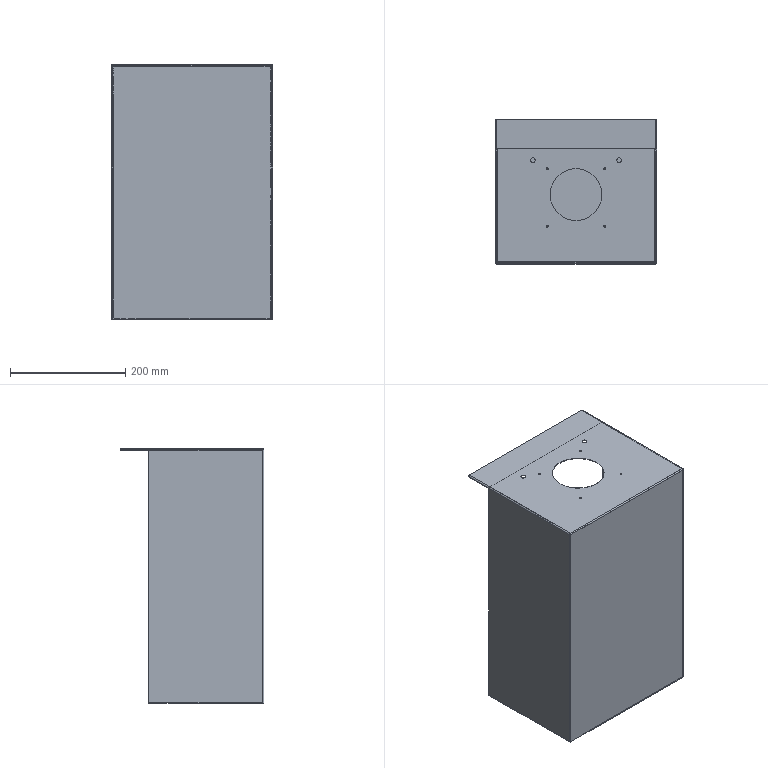Part | NX | 1 solid | 50 faces | box 280 x 250 x 443 mm | volume 446416 mm3 | cylinder 24 | plane 14 | cone 8 | sphere 4 | commonest cylinder face diameters 4 x10 2.5 x8 8.2 x4 90 x2
STEP:
#1=CARTESIAN_POINT('',(140.,100.,447.));
#2=VERTEX_POINT('',#1);
#3=CARTESIAN_POINT('',(140.,100.,7.));
#4=VERTEX_POINT('',#3);
#5=CARTESIAN_POINT('',(140.,100.,0.));
#6=DIRECTION('',(0.,0.,-1.));
#7=VECTOR('',#6,1000.);
#8=LINE('',#5,#7);
#9=EDGE_CURVE('',#2,#4,#8,.T.);
#10=ORIENTED_EDGE('',*,*,#9,.T.);
#11=CARTESIAN_POINT('',(-140.,100.,7.));
#12=VERTEX_POINT('',#11);
#13=CARTESIAN_POINT('',(0.,100.,7.));
#14=DIRECTION('',(-1.,0.,0.));
#15=VECTOR('',#14,1000.);
#16=LINE('',#13,#15);
#17=EDGE_CURVE('',#4,#12,#16,.T.);
#18=ORIENTED_EDGE('',*,*,#17,.T.);
#19=CARTESIAN_POINT('',(-140.,100.,447.));
#20=VERTEX_POINT('',#19);
#21=CARTESIAN_POINT('',(-140.,100.,0.));
#22=DIRECTION('',(0.,0.,-1.));
#23=VECTOR('',#22,1000.);
#24=LINE('',#21,#23);
#25=EDGE_CURVE('',#20,#12,#24,.T.);
#26=ORIENTED_EDGE('',*,*,#25,.F.);
#27=CARTESIAN_POINT('',(-139.,100.,447.));
#28=VERTEX_POINT('',#27);
#29=CARTESIAN_POINT('',(-140.,100.,447.));
#30=DIRECTION('',(1.,0.,0.));
#31=VECTOR('',#30,1000.);
#32=LINE('',#29,#31);
#33=EDGE_CURVE('',#20,#28,#32,.T.);
#34=ORIENTED_EDGE('',*,*,#33,.T.);
#35=CARTESIAN_POINT('',(-139.,100.,8.));
#36=VERTEX_POINT('',#35);
#37=CARTESIAN_POINT('',(-139.,100.,0.));
#38=DIRECTION('',(0.,0.,-1.));
#39=VECTOR('',#38,1000.);
#40=LINE('',#37,#39);
#41=EDGE_CURVE('',#28,#36,#40,.T.);
#42=ORIENTED_EDGE('',*,*,#41,.T.);
#43=CARTESIAN_POINT('',(139.,100.,8.));
#44=VERTEX_POINT('',#43);
#45=CARTESIAN_POINT('',(0.,100.,8.));
#46=DIRECTION('',(-1.,0.,0.));
#47=VECTOR('',#46,1000.);
#48=LINE('',#45,#47);
#49=EDGE_CURVE('',#44,#36,#48,.T.);
#50=ORIENTED_EDGE('',*,*,#49,.F.);
#51=CARTESIAN_POINT('',(139.,100.,447.));
#52=VERTEX_POINT('',#51);
#53=CARTESIAN_POINT('',(139.,100.,0.));
#54=DIRECTION('',(0.,0.,-1.));
#55=VECTOR('',#54,1000.);
#56=LINE('',#53,#55);
#57=EDGE_CURVE('',#52,#44,#56,.T.);
#58=ORIENTED_EDGE('',*,*,#57,.F.);
#59=CARTESIAN_POINT('',(139.,100.,447.));
#60=DIRECTION('',(1.,0.,0.));
#61=VECTOR('',#60,1000.);
#62=LINE('',#59,#61);
#63=EDGE_CURVE('',#52,#2,#62,.T.);
#64=ORIENTED_EDGE('',*,*,#63,.T.);
#65=EDGE_LOOP('',(#10,#18,#26,#34,#42,#50,#58,#64));
#66=FACE_BOUND('',#65,.T.);
#67=CARTESIAN_POINT('',(140.,100.,0.));
#68=DIRECTION('',(0.,1.,0.));
#69=DIRECTION('',(1.,0.,0.));
#70=AXIS2_PLACEMENT_3D('',#67,#68,#69);
#71=PLANE('',#70);
#72=ADVANCED_FACE('',(#66),#71,.T.);
#73=ORIENTED_EDGE('',*,*,#63,.F.);
#74=CARTESIAN_POINT('',(-139.,100.,447.));
#75=DIRECTION('',(1.,0.,0.));
#76=VECTOR('',#75,1000.);
#77=LINE('',#74,#76);
#78=EDGE_CURVE('',#28,#52,#77,.T.);
#79=ORIENTED_EDGE('',*,*,#78,.F.);
#80=ORIENTED_EDGE('',*,*,#33,.F.);
#81=CARTESIAN_POINT('',(-140.,150.,447.));
#82=VERTEX_POINT('',#81);
#83=CARTESIAN_POINT('',(-140.,150.,447.));
#84=DIRECTION('',(0.,-1.,0.));
#85=VECTOR('',#84,1000.);
#86=LINE('',#83,#85);
#87=EDGE_CURVE('',#82,#20,#86,.T.);
#88=ORIENTED_EDGE('',*,*,#87,.F.);
#89=CARTESIAN_POINT('',(140.,150.,447.));
#90=VERTEX_POINT('',#89);
#91=CARTESIAN_POINT('',(-140.,150.,447.));
#92=DIRECTION('',(1.,0.,0.));
#93=VECTOR('',#92,1000.);
#94=LINE('',#91,#93);
#95=EDGE_CURVE('',#82,#90,#94,.T.);
#96=ORIENTED_EDGE('',*,*,#95,.T.);
#97=CARTESIAN_POINT('',(140.,150.,447.));
#98=DIRECTION('',(0.,-1.,0.));
#99=VECTOR('',#98,1000.);
#100=LINE('',#97,#99);
#101=EDGE_CURVE('',#90,#2,#100,.T.);
#102=ORIENTED_EDGE('',*,*,#101,.T.);
#103=EDGE_LOOP('',(#73,#79,#80,#88,#96,#102));
#104=FACE_BOUND('',#103,.T.);
#105=CARTESIAN_POINT('',(140.,100.,447.));
#106=DIRECTION('',(0.,0.,-1.));
#107=DIRECTION('',(0.,-1.,0.));
#108=AXIS2_PLACEMENT_3D('',#105,#106,#107);
#109=PLANE('',#108);
#110=ADVANCED_FACE('',(#104),#109,.T.);
#111=CARTESIAN_POINT('',(-139.,-97.,447.));
#112=VERTEX_POINT('',#111);
#113=CARTESIAN_POINT('',(-139.,100.,447.));
#114=DIRECTION('',(0.,-1.,0.));
#115=VECTOR('',#114,1000.);
#116=LINE('',#113,#115);
#117=EDGE_CURVE('',#28,#112,#116,.T.);
#118=ORIENTED_EDGE('',*,*,#117,.T.);
#119=CARTESIAN_POINT('',(-139.,-97.,8.));
#120=VERTEX_POINT('',#119);
#121=CARTESIAN_POINT('',(-139.,-97.,447.));
#122=DIRECTION('',(0.,0.,-1.));
#123=VECTOR('',#122,1000.);
#124=LINE('',#121,#123);
#125=EDGE_CURVE('',#112,#120,#124,.T.);
#126=ORIENTED_EDGE('',*,*,#125,.T.);
#127=CARTESIAN_POINT('',(-139.,0.,8.));
#128=DIRECTION('',(0.,-1.,0.));
#129=VECTOR('',#128,1000.);
#130=LINE('',#127,#129);
#131=EDGE_CURVE('',#36,#120,#130,.T.);
#132=ORIENTED_EDGE('',*,*,#131,.F.);
#133=ORIENTED_EDGE('',*,*,#41,.F.);
#134=EDGE_LOOP('',(#118,#126,#132,#133));
#135=FACE_BOUND('',#134,.T.);
#136=CARTESIAN_POINT('',(-139.,100.,0.));
#137=DIRECTION('',(-1.,0.,0.));
#138=DIRECTION('',(0.,0.,1.));
#139=AXIS2_PLACEMENT_3D('',#136,#137,#138);
#140=PLANE('',#139);
#141=ADVANCED_FACE('',(#135),#140,.F.);
#142=CARTESIAN_POINT('',(139.,-97.,447.));
#143=VERTEX_POINT('',#142);
#144=CARTESIAN_POINT('',(139.,-97.,447.));
#145=DIRECTION('',(0.,1.,0.));
#146=VECTOR('',#145,1000.);
#147=LINE('',#144,#146);
#148=EDGE_CURVE('',#143,#52,#147,.T.);
#149=ORIENTED_EDGE('',*,*,#148,.T.);
#150=ORIENTED_EDGE('',*,*,#57,.T.);
#151=CARTESIAN_POINT('',(139.,-97.,8.));
#152=VERTEX_POINT('',#151);
#153=CARTESIAN_POINT('',(139.,0.,8.));
#154=DIRECTION('',(0.,1.,0.));
#155=VECTOR('',#154,1000.);
#156=LINE('',#153,#155);
#157=EDGE_CURVE('',#152,#44,#156,.T.);
#158=ORIENTED_EDGE('',*,*,#157,.F.);
#159=CARTESIAN_POINT('',(139.,-97.,3.));
#160=DIRECTION('',(0.,0.,1.));
#161=VECTOR('',#160,1000.);
#162=LINE('',#159,#161);
#163=EDGE_CURVE('',#152,#143,#162,.T.);
#164=ORIENTED_EDGE('',*,*,#163,.T.);
#165=EDGE_LOOP('',(#149,#150,#158,#164));
#166=FACE_BOUND('',#165,.T.);
#167=CARTESIAN_POINT('',(139.,-100.,0.));
#168=DIRECTION('',(1.,0.,0.));
#169=DIRECTION('',(0.,1.,0.));
#170=AXIS2_PLACEMENT_3D('',#167,#168,#169);
#171=PLANE('',#170);
#172=ADVANCED_FACE('',(#166),#171,.F.);
#173=CARTESIAN_POINT('',(137.,100.,449.));
#174=VERTEX_POINT('',#173);
#175=CARTESIAN_POINT('',(137.,100.,447.));
#176=DIRECTION('',(0.,1.,0.));
#177=DIRECTION('',(0.,0.,1.));
#178=AXIS2_PLACEMENT_3D('',#175,#176,#177);
#179=CIRCLE('',#178,2.);
#180=EDGE_CURVE('',#174,#52,#179,.T.);
#181=ORIENTED_EDGE('',*,*,#180,.T.);
#182=ORIENTED_EDGE('',*,*,#148,.F.);
#183=CARTESIAN_POINT('',(137.,-97.,449.));
#184=VERTEX_POINT('',#183);
#185=CARTESIAN_POINT('',(137.,-97.,447.));
#186=DIRECTION('',(0.,1.,0.));
#187=DIRECTION('',(1.,0.,0.));
#188=AXIS2_PLACEMENT_3D('',#185,#186,#187);
#189=CIRCLE('',#188,2.);
#190=EDGE_CURVE('',#184,#143,#189,.T.);
#191=ORIENTED_EDGE('',*,*,#190,.F.);
#192=CARTESIAN_POINT('',(137.,100.,449.));
#193=DIRECTION('',(0.,-1.,0.));
#194=VECTOR('',#193,1000.);
#195=LINE('',#192,#194);
#196=EDGE_CURVE('',#174,#184,#195,.T.);
#197=ORIENTED_EDGE('',*,*,#196,.F.);
#198=EDGE_LOOP('',(#181,#182,#191,#197));
#199=FACE_BOUND('',#198,.T.);
#200=CARTESIAN_POINT('',(137.,-99.854,447.));
#201=DIRECTION('',(0.,1.,0.));
#202=DIRECTION('',(0.,0.,1.));
#203=AXIS2_PLACEMENT_3D('',#200,#201,#202);
#204=CYLINDRICAL_SURFACE('',#203,2.);
#205=ADVANCED_FACE('',(#199),#204,.F.);
#206=CARTESIAN_POINT('',(138.,-100.,7.));
#207=VERTEX_POINT('',#206);
#208=CARTESIAN_POINT('',(138.,-100.,448.));
#209=VERTEX_POINT('',#208);
#210=CARTESIAN_POINT('',(138.,-100.,2.));
#211=DIRECTION('',(0.,0.,1.));
#212=VECTOR('',#211,1000.);
#213=LINE('',#210,#212);
#214=EDGE_CURVE('',#207,#209,#213,.T.);
#215=ORIENTED_EDGE('',*,*,#214,.F.);
#216=CARTESIAN_POINT('',(140.,-98.,7.));
#217=VERTEX_POINT('',#216);
#218=CARTESIAN_POINT('',(138.,-98.,7.));
#219=DIRECTION('',(0.,0.,-1.));
#220=DIRECTION('',(1.,0.,0.));
#221=AXIS2_PLACEMENT_3D('',#218,#219,#220);
#222=CIRCLE('',#221,2.);
#223=EDGE_CURVE('',#217,#207,#222,.T.);
#224=ORIENTED_EDGE('',*,*,#223,.F.);
#225=CARTESIAN_POINT('',(140.,-98.,448.));
#226=VERTEX_POINT('',#225);
#227=CARTESIAN_POINT('',(140.,-98.,448.));
#228=DIRECTION('',(0.,0.,-1.));
#229=VECTOR('',#228,1000.);
#230=LINE('',#227,#229);
#231=EDGE_CURVE('',#226,#217,#230,.T.);
#232=ORIENTED_EDGE('',*,*,#231,.F.);
#233=CARTESIAN_POINT('',(138.,-98.,448.));
#234=DIRECTION('',(0.,0.,-1.));
#235=DIRECTION('',(1.,0.,0.));
#236=AXIS2_PLACEMENT_3D('',#233,#234,#235);
#237=CIRCLE('',#236,2.);
#238=EDGE_CURVE('',#226,#209,#237,.T.);
#239=ORIENTED_EDGE('',*,*,#238,.T.);
#240=EDGE_LOOP('',(#215,#224,#232,#239));
#241=FACE_BOUND('',#240,.T.);
#242=CARTESIAN_POINT('',(138.,-98.,450.886));
#243=DIRECTION('',(0.,0.,-1.));
#244=DIRECTION('',(1.,0.,0.));
#245=AXIS2_PLACEMENT_3D('',#242,#243,#244);
#246=CYLINDRICAL_SURFACE('',#245,2.);
#247=ADVANCED_FACE('',(#241),#246,.T.);
#248=CARTESIAN_POINT('',(-140.,-98.,7.));
#249=VERTEX_POINT('',#248);
#250=CARTESIAN_POINT('',(-140.,-98.,448.));
#251=VERTEX_POINT('',#250);
#252=CARTESIAN_POINT('',(-140.,-98.,2.));
#253=DIRECTION('',(0.,0.,1.));
#254=VECTOR('',#253,1000.);
#255=LINE('',#252,#254);
#256=EDGE_CURVE('',#249,#251,#255,.T.);
#257=ORIENTED_EDGE('',*,*,#256,.F.);
#258=CARTESIAN_POINT('',(-138.,-100.,7.));
#259=VERTEX_POINT('',#258);
#260=CARTESIAN_POINT('',(-138.,-98.,7.));
#261=DIRECTION('',(0.,0.,-1.));
#262=DIRECTION('',(0.,-1.,0.));
#263=AXIS2_PLACEMENT_3D('',#260,#261,#262);
#264=CIRCLE('',#263,2.);
#265=EDGE_CURVE('',#259,#249,#264,.T.);
#266=ORIENTED_EDGE('',*,*,#265,.F.);
#267=CARTESIAN_POINT('',(-138.,-100.,448.));
#268=VERTEX_POINT('',#267);
#269=CARTESIAN_POINT('',(-138.,-100.,448.));
#270=DIRECTION('',(0.,0.,-1.));
#271=VECTOR('',#270,1000.);
#272=LINE('',#269,#271);
#273=EDGE_CURVE('',#268,#259,#272,.T.);
#274=ORIENTED_EDGE('',*,*,#273,.F.);
#275=CARTESIAN_POINT('',(-138.,-98.,448.));
#276=DIRECTION('',(0.,0.,-1.));
#277=DIRECTION('',(0.,-1.,0.));
#278=AXIS2_PLACEMENT_3D('',#275,#276,#277);
#279=CIRCLE('',#278,2.);
#280=EDGE_CURVE('',#268,#251,#279,.T.);
#281=ORIENTED_EDGE('',*,*,#280,.T.);
#282=EDGE_LOOP('',(#257,#266,#274,#281));
#283=FACE_BOUND('',#282,.T.);
#284=CARTESIAN_POINT('',(-138.,-98.,450.886));
#285=DIRECTION('',(0.,0.,-1.));
#286=DIRECTION('',(0.,-1.,0.));
#287=AXIS2_PLACEMENT_3D('',#284,#285,#286);
#288=CYLINDRICAL_SURFACE('',#287,2.);
#289=ADVANCED_FACE('',(#283),#288,.T.);
#290=CARTESIAN_POINT('',(-138.,-98.,450.));
#291=VERTEX_POINT('',#290);
#292=CARTESIAN_POINT('',(-138.,-98.,448.));
#293=DIRECTION('',(1.,0.,0.));
#294=DIRECTION('',(0.,0.,1.));
#295=AXIS2_PLACEMENT_3D('',#292,#293,#294);
#296=CIRCLE('',#295,2.);
#297=EDGE_CURVE('',#291,#268,#296,.T.);
#298=ORIENTED_EDGE('',*,*,#297,.F.);
#299=CARTESIAN_POINT('',(-138.,-98.,448.));
#300=DIRECTION('',(0.,1.,0.));
#301=DIRECTION('',(1.,0.,0.));
#302=AXIS2_PLACEMENT_3D('',#299,#300,#301);
#303=CIRCLE('',#302,2.);
#304=EDGE_CURVE('',#251,#291,#303,.T.);
#305=ORIENTED_EDGE('',*,*,#304,.F.);
#306=ORIENTED_EDGE('',*,*,#280,.F.);
#307=EDGE_LOOP('',(#298,#305,#306));
#308=FACE_BOUND('',#307,.T.);
#309=CARTESIAN_POINT('',(-138.,-98.,448.));
#310=DIRECTION('',(0.,1.,0.));
#311=DIRECTION('',(1.,0.,0.));
#312=AXIS2_PLACEMENT_3D('',#309,#310,#311);
#313=SPHERICAL_SURFACE('',#312,2.);
#314=ADVANCED_FACE('',(#308),#313,.T.);
#315=CARTESIAN_POINT('',(-140.,150.,448.));
#316=VERTEX_POINT('',#315);
#317=CARTESIAN_POINT('',(-140.,-98.,448.));
#318=DIRECTION('',(0.,1.,0.));
#319=VECTOR('',#318,1000.);
#320=LINE('',#317,#319);
#321=EDGE_CURVE('',#251,#316,#320,.T.);
#322=ORIENTED_EDGE('',*,*,#321,.F.);
#323=ORIENTED_EDGE('',*,*,#304,.T.);
#324=CARTESIAN_POINT('',(-138.,150.,450.));
#325=VERTEX_POINT('',#324);
#326=CARTESIAN_POINT('',(-138.,150.,450.));
#327=DIRECTION('',(0.,-1.,0.));
#328=VECTOR('',#327,1000.);
#329=LINE('',#326,#328);
#330=EDGE_CURVE('',#325,#291,#329,.T.);
#331=ORIENTED_EDGE('',*,*,#330,.F.);
#332=CARTESIAN_POINT('',(-138.,150.,448.));
#333=DIRECTION('',(0.,-1.,0.));
#334=DIRECTION('',(0.,0.,1.));
#335=AXIS2_PLACEMENT_3D('',#332,#333,#334);
#336=CIRCLE('',#335,2.);
#337=EDGE_CURVE('',#325,#316,#336,.T.);
#338=ORIENTED_EDGE('',*,*,#337,.T.);
#339=EDGE_LOOP('',(#322,#323,#331,#338));
#340=FACE_BOUND('',#339,.T.);
#341=CARTESIAN_POINT('',(-138.,100.871,448.));
#342=DIRECTION('',(0.,-1.,0.));
#343=DIRECTION('',(0.,0.,1.));
#344=AXIS2_PLACEMENT_3D('',#341,#342,#343);
#345=CYLINDRICAL_SURFACE('',#344,2.);
#346=ADVANCED_FACE('',(#340),#345,.T.);
#347=CARTESIAN_POINT('',(140.,150.,448.));
#348=VERTEX_POINT('',#347);
#349=CARTESIAN_POINT('',(138.,150.,450.));
#350=VERTEX_POINT('',#349);
#351=CARTESIAN_POINT('',(138.,150.,448.));
#352=DIRECTION('',(0.,-1.,0.));
#353=DIRECTION('',(1.,0.,0.));
#354=AXIS2_PLACEMENT_3D('',#351,#352,#353);
#355=CIRCLE('',#354,2.);
#356=EDGE_CURVE('',#348,#350,#355,.T.);
#357=ORIENTED_EDGE('',*,*,#356,.F.);
#358=CARTESIAN_POINT('',(140.,150.,447.));
#359=DIRECTION('',(0.,0.,1.));
#360=VECTOR('',#359,1000.);
#361=LINE('',#358,#360);
#362=EDGE_CURVE('',#90,#348,#361,.T.);
#363=ORIENTED_EDGE('',*,*,#362,.F.);
#364=ORIENTED_EDGE('',*,*,#95,.F.);
#365=CARTESIAN_POINT('',(-140.,150.,448.));
#366=DIRECTION('',(0.,0.,-1.));
#367=VECTOR('',#366,1000.);
#368=LINE('',#365,#367);
#369=EDGE_CURVE('',#316,#82,#368,.T.);
#370=ORIENTED_EDGE('',*,*,#369,.F.);
#371=ORIENTED_EDGE('',*,*,#337,.F.);
#372=CARTESIAN_POINT('',(0.,150.,450.));
#373=DIRECTION('',(1.,0.,0.));
#374=VECTOR('',#373,1000.);
#375=LINE('',#372,#374);
#376=EDGE_CURVE('',#325,#350,#375,.T.);
#377=ORIENTED_EDGE('',*,*,#376,.T.);
#378=EDGE_LOOP('',(#357,#363,#364,#370,#371,#377));
#379=FACE_BOUND('',#378,.T.);
#380=CARTESIAN_POINT('',(0.,150.,0.));
#381=DIRECTION('',(0.,1.,0.));
#382=DIRECTION('',(1.,0.,0.));
#383=AXIS2_PLACEMENT_3D('',#380,#381,#382);
#384=PLANE('',#383);
#385=ADVANCED_FACE('',(#379),#384,.T.);
#386=CARTESIAN_POINT('',(138.,-98.,450.));
#387=VERTEX_POINT('',#386);
#388=CARTESIAN_POINT('',(-138.,-98.,450.));
#389=DIRECTION('',(1.,0.,0.));
#390=VECTOR('',#389,1000.);
#391=LINE('',#388,#390);
#392=EDGE_CURVE('',#291,#387,#391,.T.);
#393=ORIENTED_EDGE('',*,*,#392,.F.);
#394=ORIENTED_EDGE('',*,*,#297,.T.);
#395=CARTESIAN_POINT('',(138.,-100.,448.));
#396=DIRECTION('',(-1.,0.,0.));
#397=VECTOR('',#396,1000.);
#398=LINE('',#395,#397);
#399=EDGE_CURVE('',#209,#268,#398,.T.);
#400=ORIENTED_EDGE('',*,*,#399,.F.);
#401=CARTESIAN_POINT('',(138.,-98.,448.));
#402=DIRECTION('',(-1.,0.,0.));
#403=DIRECTION('',(0.,-1.,0.));
#404=AXIS2_PLACEMENT_3D('',#401,#402,#403);
#405=CIRCLE('',#404,2.);
#406=EDGE_CURVE('',#209,#387,#405,.T.);
#407=ORIENTED_EDGE('',*,*,#406,.T.);
#408=EDGE_LOOP('',(#393,#394,#400,#407));
#409=FACE_BOUND('',#408,.T.);
#410=CARTESIAN_POINT('',(-140.871,-98.,448.));
#411=DIRECTION('',(1.,0.,0.));
#412=DIRECTION('',(0.,0.,1.));
#413=AXIS2_PLACEMENT_3D('',#410,#411,#412);
#414=CYLINDRICAL_SURFACE('',#413,2.);
#415=ADVANCED_FACE('',(#409),#414,.T.);
#416=CARTESIAN_POINT('',(138.,-98.,448.));
#417=DIRECTION('',(0.,1.,0.));
#418=DIRECTION('',(1.,0.,0.));
#419=AXIS2_PLACEMENT_3D('',#416,#417,#418);
#420=CIRCLE('',#419,2.);
#421=EDGE_CURVE('',#387,#226,#420,.T.);
#422=ORIENTED_EDGE('',*,*,#421,.F.);
#423=ORIENTED_EDGE('',*,*,#406,.F.);
#424=ORIENTED_EDGE('',*,*,#238,.F.);
#425=EDGE_LOOP('',(#422,#423,#424));
#426=FACE_BOUND('',#425,.T.);
#427=CARTESIAN_POINT('',(138.,-98.,448.));
#428=DIRECTION('',(0.,1.,0.));
#429=DIRECTION('',(1.,0.,0.));
#430=AXIS2_PLACEMENT_3D('',#427,#428,#429);
#431=SPHERICAL_SURFACE('',#430,2.);
#432=ADVANCED_FACE('',(#426),#431,.T.);
#433=CARTESIAN_POINT('',(138.,-98.,450.));
#434=DIRECTION('',(0.,1.,0.));
#435=VECTOR('',#434,1000.);
#436=LINE('',#433,#435);
#437=EDGE_CURVE('',#387,#350,#436,.T.);
#438=ORIENTED_EDGE('',*,*,#437,.F.);
#439=ORIENTED_EDGE('',*,*,#421,.T.);
#440=CARTESIAN_POINT('',(140.,150.,448.));
#441=DIRECTION('',(0.,-1.,0.));
#442=VECTOR('',#441,1000.);
#443=LINE('',#440,#442);
#444=EDGE_CURVE('',#348,#226,#443,.T.);
#445=ORIENTED_EDGE('',*,*,#444,.F.);
#446=ORIENTED_EDGE('',*,*,#356,.T.);
#447=EDGE_LOOP('',(#438,#439,#445,#446));
#448=FACE_BOUND('',#447,.T.);
#449=CARTESIAN_POINT('',(138.,-100.854,448.));
#450=DIRECTION('',(0.,1.,0.));
#451=DIRECTION('',(0.,0.,1.));
#452=AXIS2_PLACEMENT_3D('',#449,#450,#451);
#453=CYLINDRICAL_SURFACE('',#452,2.);
#454=ADVANCED_FACE('',(#448),#453,.T.);
#455=CARTESIAN_POINT('',(-137.,-99.,8.));
#456=VERTEX_POINT('',#455);
#457=CARTESIAN_POINT('',(-137.,-97.,8.));
#458=DIRECTION('',(0.,0.,-1.));
#459=DIRECTION('',(0.,-1.,0.));
#460=AXIS2_PLACEMENT_3D('',#457,#458,#459);
#461=CIRCLE('',#460,2.);
#462=EDGE_CURVE('',#456,#120,#461,.T.);
#463=ORIENTED_EDGE('',*,*,#462,.T.);
#464=ORIENTED_EDGE('',*,*,#125,.F.);
#465=CARTESIAN_POINT('',(-137.,-99.,447.));
#466=VERTEX_POINT('',#465);
#467=CARTESIAN_POINT('',(-137.,-97.,447.));
#468=DIRECTION('',(0.,0.,1.));
#469=DIRECTION('',(-1.,0.,0.));
#470=AXIS2_PLACEMENT_3D('',#467,#468,#469);
#471=CIRCLE('',#470,2.);
#472=EDGE_CURVE('',#112,#466,#471,.T.);
#473=ORIENTED_EDGE('',*,*,#472,.T.);
#474=CARTESIAN_POINT('',(-137.,-99.,3.));
#475=DIRECTION('',(0.,0.,1.));
#476=VECTOR('',#475,1000.);
#477=LINE('',#474,#476);
#478=EDGE_CURVE('',#456,#466,#477,.T.);
#479=ORIENTED_EDGE('',*,*,#478,.F.);
#480=EDGE_LOOP('',(#463,#464,#473,#479));
#481=FACE_BOUND('',#480,.T.);
#482=CARTESIAN_POINT('',(-137.,-97.,449.886));
#483=DIRECTION('',(0.,0.,-1.));
#484=DIRECTION('',(0.,-1.,0.));
#485=AXIS2_PLACEMENT_3D('',#482,#483,#484);
#486=CYLINDRICAL_SURFACE('',#485,2.);
#487=ADVANCED_FACE('',(#481),#486,.F.);
#488=ORIENTED_EDGE('',*,*,#17,.F.);
#489=CARTESIAN_POINT('',(140.,0.,7.));
#490=DIRECTION('',(0.,1.,0.));
#491=VECTOR('',#490,1000.);
#492=LINE('',#489,#491);
#493=EDGE_CURVE('',#217,#4,#492,.T.);
#494=ORIENTED_EDGE('',*,*,#493,.F.);
#495=ORIENTED_EDGE('',*,*,#223,.T.);
#496=CARTESIAN_POINT('',(0.,-100.,7.));
#497=DIRECTION('',(1.,0.,0.));
#498=VECTOR('',#497,1000.);
#499=LINE('',#496,#498);
#500=EDGE_CURVE('',#259,#207,#499,.T.);
#501=ORIENTED_EDGE('',*,*,#500,.F.);
#502=ORIENTED_EDGE('',*,*,#265,.T.);
#503=CARTESIAN_POINT('',(-140.,0.,7.));
#504=DIRECTION('',(0.,-1.,0.));
#505=VECTOR('',#504,1000.);
#506=LINE('',#503,#505);
#507=EDGE_CURVE('',#12,#249,#506,.T.);
#508=ORIENTED_EDGE('',*,*,#507,.F.);
#509=EDGE_LOOP('',(#488,#494,#495,#501,#502,#508));
#510=FACE_BOUND('',#509,.T.);
#511=CARTESIAN_POINT('',(139.524,-95.032,7.));
#512=DIRECTION('',(0.,0.,-1.));
#513=DIRECTION('',(0.,-1.,0.));
#514=AXIS2_PLACEMENT_3D('',#511,#512,#513);
#515=PLANE('',#514);
#516=ADVANCED_FACE('',(#510),#515,.T.);
#517=CARTESIAN_POINT('',(137.,-99.,8.));
#518=VERTEX_POINT('',#517);
#519=CARTESIAN_POINT('',(137.,-97.,8.));
#520=DIRECTION('',(0.,0.,-1.));
#521=DIRECTION('',(1.,0.,0.));
#522=AXIS2_PLACEMENT_3D('',#519,#520,#521);
#523=CIRCLE('',#522,2.);
#524=EDGE_CURVE('',#152,#518,#523,.T.);
#525=ORIENTED_EDGE('',*,*,#524,.T.);
#526=CARTESIAN_POINT('',(137.,-99.,447.));
#527=VERTEX_POINT('',#526);
#528=CARTESIAN_POINT('',(137.,-99.,447.));
#529=DIRECTION('',(0.,0.,-1.));
#530=VECTOR('',#529,1000.);
#531=LINE('',#528,#530);
#532=EDGE_CURVE('',#527,#518,#531,.T.);
#533=ORIENTED_EDGE('',*,*,#532,.F.);
#534=CARTESIAN_POINT('',(137.,-97.,447.));
#535=DIRECTION('',(0.,0.,1.));
#536=DIRECTION('',(0.,-1.,0.));
#537=AXIS2_PLACEMENT_3D('',#534,#535,#536);
#538=CIRCLE('',#537,2.);
#539=EDGE_CURVE('',#527,#143,#538,.T.);
#540=ORIENTED_EDGE('',*,*,#539,.T.);
#541=ORIENTED_EDGE('',*,*,#163,.F.);
#542=EDGE_LOOP('',(#525,#533,#540,#541));
#543=FACE_BOUND('',#542,.T.);
#544=CARTESIAN_POINT('',(137.,-97.,449.886));
#545=DIRECTION('',(0.,0.,-1.));
#546=DIRECTION('',(1.,0.,0.));
#547=AXIS2_PLACEMENT_3D('',#544,#545,#546);
#548=CYLINDRICAL_SURFACE('',#547,2.);
#549=ADVANCED_FACE('',(#543),#548,.F.);
#550=ORIENTED_EDGE('',*,*,#478,.T.);
#551=CARTESIAN_POINT('',(-137.,-99.,447.));
#552=DIRECTION('',(1.,0.,0.));
#553=VECTOR('',#552,1000.);
#554=LINE('',#551,#553);
#555=EDGE_CURVE('',#466,#527,#554,.T.);
#556=ORIENTED_EDGE('',*,*,#555,.T.);
#557=ORIENTED_EDGE('',*,*,#532,.T.);
#558=CARTESIAN_POINT('',(0.,-99.,8.));
#559=DIRECTION('',(1.,0.,0.));
#560=VECTOR('',#559,1000.);
#561=LINE('',#558,#560);
#562=EDGE_CURVE('',#456,#518,#561,.T.);
#563=ORIENTED_EDGE('',*,*,#562,.F.);
#564=EDGE_LOOP('',(#550,#556,#557,#563));
#565=FACE_BOUND('',#564,.T.);
#566=CARTESIAN_POINT('',(-140.,-99.,0.));
#567=DIRECTION('',(0.,-1.,0.));
#568=DIRECTION('',(0.,0.,-1.));
#569=AXIS2_PLACEMENT_3D('',#566,#567,#568);
#570=PLANE('',#569);
#571=ADVANCED_FACE('',(#565),#570,.F.);
#572=CARTESIAN_POINT('',(-137.,-97.,449.));
#573=VERTEX_POINT('',#572);
#574=CARTESIAN_POINT('',(137.,-97.,449.));
#575=DIRECTION('',(-1.,0.,0.));
#576=VECTOR('',#575,1000.);
#577=LINE('',#574,#576);
#578=EDGE_CURVE('',#184,#573,#577,.T.);
#579=ORIENTED_EDGE('',*,*,#578,.F.);
#580=CARTESIAN_POINT('',(137.,-97.,447.));
#581=DIRECTION('',(1.,0.,0.));
#582=DIRECTION('',(0.,0.,1.));
#583=AXIS2_PLACEMENT_3D('',#580,#581,#582);
#584=CIRCLE('',#583,2.);
#585=EDGE_CURVE('',#184,#527,#584,.T.);
#586=ORIENTED_EDGE('',*,*,#585,.T.);
#587=ORIENTED_EDGE('',*,*,#555,.F.);
#588=CARTESIAN_POINT('',(-137.,-97.,447.));
#589=DIRECTION('',(-1.,0.,0.));
#590=DIRECTION('',(0.,-1.,0.));
#591=AXIS2_PLACEMENT_3D('',#588,#589,#590);
#592=CIRCLE('',#591,2.);
#593=EDGE_CURVE('',#466,#573,#592,.T.);
#594=ORIENTED_EDGE('',*,*,#593,.T.);
#595=EDGE_LOOP('',(#579,#586,#587,#594));
#596=FACE_BOUND('',#595,.T.);
#597=CARTESIAN_POINT('',(-139.871,-97.,447.));
#598=DIRECTION('',(1.,0.,0.));
#599=DIRECTION('',(0.,0.,1.));
#600=AXIS2_PLACEMENT_3D('',#597,#598,#599);
#601=CYLINDRICAL_SURFACE('',#600,2.);
#602=ADVANCED_FACE('',(#596),#601,.F.);
#603=ORIENTED_EDGE('',*,*,#593,.F.);
#604=ORIENTED_EDGE('',*,*,#472,.F.);
#605=CARTESIAN_POINT('',(-137.,-97.,447.));
#606=DIRECTION('',(0.,1.,0.));
#607=DIRECTION('',(1.,0.,0.));
#608=AXIS2_PLACEMENT_3D('',#605,#606,#607);
#609=CIRCLE('',#608,2.);
#610=EDGE_CURVE('',#112,#573,#609,.T.);
#611=ORIENTED_EDGE('',*,*,#610,.T.);
#612=EDGE_LOOP('',(#603,#604,#611));
#613=FACE_BOUND('',#612,.T.);
#614=CARTESIAN_POINT('',(-137.,-97.,447.));
#615=DIRECTION('',(0.,1.,0.));
#616=DIRECTION('',(1.,0.,0.));
#617=AXIS2_PLACEMENT_3D('',#614,#615,#616);
#618=SPHERICAL_SURFACE('',#617,2.);
#619=ADVANCED_FACE('',(#613),#618,.F.);
#620=ORIENTED_EDGE('',*,*,#131,.T.);
#621=ORIENTED_EDGE('',*,*,#462,.F.);
#622=ORIENTED_EDGE('',*,*,#562,.T.);
#623=ORIENTED_EDGE('',*,*,#524,.F.);
#624=ORIENTED_EDGE('',*,*,#157,.T.);
#625=ORIENTED_EDGE('',*,*,#49,.T.);
#626=EDGE_LOOP('',(#620,#621,#622,#623,#624,#625));
#627=FACE_BOUND('',#626,.T.);
#628=CARTESIAN_POINT('',(139.524,-95.032,8.));
#629=DIRECTION('',(0.,0.,-1.));
#630=DIRECTION('',(0.,-1.,0.));
#631=AXIS2_PLACEMENT_3D('',#628,#629,#630);
#632=PLANE('',#631);
#633=ADVANCED_FACE('',(#627),#632,.F.);
#634=ORIENTED_EDGE('',*,*,#539,.F.);
#635=ORIENTED_EDGE('',*,*,#585,.F.);
#636=ORIENTED_EDGE('',*,*,#190,.T.);
#637=EDGE_LOOP('',(#634,#635,#636));
#638=FACE_BOUND('',#637,.T.);
#639=CARTESIAN_POINT('',(137.,-97.,447.));
#640=DIRECTION('',(0.,1.,0.));
#641=DIRECTION('',(1.,0.,0.));
#642=AXIS2_PLACEMENT_3D('',#639,#640,#641);
#643=SPHERICAL_SURFACE('',#642,2.);
#644=ADVANCED_FACE('',(#638),#643,.F.);
#645=CARTESIAN_POINT('',(-137.,100.,449.));
#646=VERTEX_POINT('',#645);
#647=CARTESIAN_POINT('',(-137.,100.,447.));
#648=DIRECTION('',(0.,1.,0.));
#649=DIRECTION('',(-1.,0.,0.));
#650=AXIS2_PLACEMENT_3D('',#647,#648,#649);
#651=CIRCLE('',#650,2.);
#652=EDGE_CURVE('',#28,#646,#651,.T.);
#653=ORIENTED_EDGE('',*,*,#652,.T.);
#654=CARTESIAN_POINT('',(-137.,-97.,449.));
#655=DIRECTION('',(0.,1.,0.));
#656=VECTOR('',#655,1000.);
#657=LINE('',#654,#656);
#658=EDGE_CURVE('',#573,#646,#657,.T.);
#659=ORIENTED_EDGE('',*,*,#658,.F.);
#660=ORIENTED_EDGE('',*,*,#610,.F.);
#661=ORIENTED_EDGE('',*,*,#117,.F.);
#662=EDGE_LOOP('',(#653,#659,#660,#661));
#663=FACE_BOUND('',#662,.T.);
#664=CARTESIAN_POINT('',(-137.,100.871,447.));
#665=DIRECTION('',(0.,-1.,0.));
#666=DIRECTION('',(0.,0.,1.));
#667=AXIS2_PLACEMENT_3D('',#664,#665,#666);
#668=CYLINDRICAL_SURFACE('',#667,2.);
#669=ADVANCED_FACE('',(#663),#668,.F.);
#670=CARTESIAN_POINT('',(0.,100.,449.));
#671=DIRECTION('',(1.,0.,0.));
#672=VECTOR('',#671,1000.);
#673=LINE('',#670,#672);
#674=EDGE_CURVE('',#646,#174,#673,.T.);
#675=ORIENTED_EDGE('',*,*,#674,.F.);
#676=ORIENTED_EDGE('',*,*,#652,.F.);
#677=ORIENTED_EDGE('',*,*,#78,.T.);
#678=ORIENTED_EDGE('',*,*,#180,.F.);
#679=EDGE_LOOP('',(#675,#676,#677,#678));
#680=FACE_BOUND('',#679,.T.);
#681=CARTESIAN_POINT('',(0.,100.,0.));
#682=DIRECTION('',(0.,1.,0.));
#683=DIRECTION('',(1.,0.,0.));
#684=AXIS2_PLACEMENT_3D('',#681,#682,#683);
#685=PLANE('',#684);
#686=ADVANCED_FACE('',(#680),#685,.F.);
#687=ORIENTED_EDGE('',*,*,#658,.T.);
#688=ORIENTED_EDGE('',*,*,#674,.T.);
#689=ORIENTED_EDGE('',*,*,#196,.T.);
#690=ORIENTED_EDGE('',*,*,#578,.T.);
#691=EDGE_LOOP('',(#687,#688,#689,#690));
#692=FACE_BOUND('',#691,.T.);
#693=CARTESIAN_POINT('',(-45.,20.,449.));
#694=VERTEX_POINT('',#693);
#695=CARTESIAN_POINT('',(45.,20.,449.));
#696=VERTEX_POINT('',#695);
#697=CARTESIAN_POINT('',(0.,20.,449.));
#698=DIRECTION('',(0.,0.,1.));
#699=DIRECTION('',(1.,0.,0.));
#700=AXIS2_PLACEMENT_3D('',#697,#698,#699);
#701=CIRCLE('',#700,45.);
#702=EDGE_CURVE('',#694,#696,#701,.T.);
#703=ORIENTED_EDGE('',*,*,#702,.T.);
#704=CARTESIAN_POINT('',(0.,20.,449.));
#705=DIRECTION('',(0.,0.,1.));
#706=DIRECTION('',(1.,0.,0.));
#707=AXIS2_PLACEMENT_3D('',#704,#705,#706);
#708=CIRCLE('',#707,45.);
#709=EDGE_CURVE('',#696,#694,#708,.T.);
#710=ORIENTED_EDGE('',*,*,#709,.T.);
#711=EDGE_LOOP('',(#703,#710));
#712=FACE_BOUND('',#711,.T.);
#713=CARTESIAN_POINT('',(-79.1,80.,449.));
#714=VERTEX_POINT('',#713);
#715=CARTESIAN_POINT('',(-70.9,80.,449.));
#716=VERTEX_POINT('',#715);
#717=CARTESIAN_POINT('',(-75.,80.,449.));
#718=DIRECTION('',(0.,0.,1.));
#719=DIRECTION('',(1.,0.,0.));
#720=AXIS2_PLACEMENT_3D('',#717,#718,#719);
#721=CIRCLE('',#720,4.1);
#722=EDGE_CURVE('',#714,#716,#721,.T.);
#723=ORIENTED_EDGE('',*,*,#722,.T.);
#724=CARTESIAN_POINT('',(-75.,80.,449.));
#725=DIRECTION('',(0.,0.,1.));
#726=DIRECTION('',(1.,0.,0.));
#727=AXIS2_PLACEMENT_3D('',#724,#725,#726);
#728=CIRCLE('',#727,4.1);
#729=EDGE_CURVE('',#716,#714,#728,.T.);
#730=ORIENTED_EDGE('',*,*,#729,.T.);
#731=EDGE_LOOP('',(#723,#730));
#732=FACE_BOUND('',#731,.T.);
#733=CARTESIAN_POINT('',(70.9,80.,449.));
#734=VERTEX_POINT('',#733);
#735=CARTESIAN_POINT('',(79.1,80.,449.));
#736=VERTEX_POINT('',#735);
#737=CARTESIAN_POINT('',(75.,80.,449.));
#738=DIRECTION('',(0.,0.,1.));
#739=DIRECTION('',(1.,0.,0.));
#740=AXIS2_PLACEMENT_3D('',#737,#738,#739);
#741=CIRCLE('',#740,4.1);
#742=EDGE_CURVE('',#734,#736,#741,.T.);
#743=ORIENTED_EDGE('',*,*,#742,.T.);
#744=CARTESIAN_POINT('',(75.,80.,449.));
#745=DIRECTION('',(0.,0.,1.));
#746=DIRECTION('',(1.,0.,0.));
#747=AXIS2_PLACEMENT_3D('',#744,#745,#746);
#748=CIRCLE('',#747,4.1);
#749=EDGE_CURVE('',#736,#734,#748,.T.);
#750=ORIENTED_EDGE('',*,*,#749,.T.);
#751=EDGE_LOOP('',(#743,#750));
#752=FACE_BOUND('',#751,.T.);
#753=CARTESIAN_POINT('',(48.75,-35.,449.));
#754=VERTEX_POINT('',#753);
#755=CARTESIAN_POINT('',(51.25,-35.,449.));
#756=VERTEX_POINT('',#755);
#757=CARTESIAN_POINT('',(50.,-35.,449.));
#758=DIRECTION('',(0.,0.,1.));
#759=DIRECTION('',(1.,0.,0.));
#760=AXIS2_PLACEMENT_3D('',#757,#758,#759);
#761=CIRCLE('',#760,1.25);
#762=EDGE_CURVE('',#754,#756,#761,.T.);
#763=ORIENTED_EDGE('',*,*,#762,.T.);
#764=CARTESIAN_POINT('',(50.,-35.,449.));
#765=DIRECTION('',(0.,0.,1.));
#766=DIRECTION('',(1.,0.,0.));
#767=AXIS2_PLACEMENT_3D('',#764,#765,#766);
#768=CIRCLE('',#767,1.25);
#769=EDGE_CURVE('',#756,#754,#768,.T.);
#770=ORIENTED_EDGE('',*,*,#769,.T.);
#771=EDGE_LOOP('',(#763,#770));
#772=FACE_BOUND('',#771,.T.);
#773=CARTESIAN_POINT('',(-51.25,-35.,449.));
#774=VERTEX_POINT('',#773);
#775=CARTESIAN_POINT('',(-48.75,-35.,449.));
#776=VERTEX_POINT('',#775);
#777=CARTESIAN_POINT('',(-50.,-35.,449.));
#778=DIRECTION('',(0.,0.,1.));
#779=DIRECTION('',(1.,0.,0.));
#780=AXIS2_PLACEMENT_3D('',#777,#778,#779);
#781=CIRCLE('',#780,1.25);
#782=EDGE_CURVE('',#774,#776,#781,.T.);
#783=ORIENTED_EDGE('',*,*,#782,.T.);
#784=CARTESIAN_POINT('',(-50.,-35.,449.));
#785=DIRECTION('',(0.,0.,1.));
#786=DIRECTION('',(1.,0.,0.));
#787=AXIS2_PLACEMENT_3D('',#784,#785,#786);
#788=CIRCLE('',#787,1.25);
#789=EDGE_CURVE('',#776,#774,#788,.T.);
#790=ORIENTED_EDGE('',*,*,#789,.T.);
#791=EDGE_LOOP('',(#783,#790));
#792=FACE_BOUND('',#791,.T.);
#793=CARTESIAN_POINT('',(-51.25,65.,449.));
#794=VERTEX_POINT('',#793);
#795=CARTESIAN_POINT('',(-48.75,65.,449.));
#796=VERTEX_POINT('',#795);
#797=CARTESIAN_POINT('',(-50.,65.,449.));
#798=DIRECTION('',(0.,0.,1.));
#799=DIRECTION('',(1.,0.,0.));
#800=AXIS2_PLACEMENT_3D('',#797,#798,#799);
#801=CIRCLE('',#800,1.25);
#802=EDGE_CURVE('',#794,#796,#801,.T.);
#803=ORIENTED_EDGE('',*,*,#802,.T.);
#804=CARTESIAN_POINT('',(-50.,65.,449.));
#805=DIRECTION('',(0.,0.,1.));
#806=DIRECTION('',(1.,0.,0.));
#807=AXIS2_PLACEMENT_3D('',#804,#805,#806);
#808=CIRCLE('',#807,1.25);
#809=EDGE_CURVE('',#796,#794,#808,.T.);
#810=ORIENTED_EDGE('',*,*,#809,.T.);
#811=EDGE_LOOP('',(#803,#810));
#812=FACE_BOUND('',#811,.T.);
#813=CARTESIAN_POINT('',(48.75,65.,449.));
#814=VERTEX_POINT('',#813);
#815=CARTESIAN_POINT('',(51.25,65.,449.));
#816=VERTEX_POINT('',#815);
#817=CARTESIAN_POINT('',(50.,65.,449.));
#818=DIRECTION('',(0.,0.,1.));
#819=DIRECTION('',(1.,0.,0.));
#820=AXIS2_PLACEMENT_3D('',#817,#818,#819);
#821=CIRCLE('',#820,1.25);
#822=EDGE_CURVE('',#814,#816,#821,.T.);
#823=ORIENTED_EDGE('',*,*,#822,.T.);
#824=CARTESIAN_POINT('',(50.,65.,449.));
#825=DIRECTION('',(0.,0.,1.));
#826=DIRECTION('',(1.,0.,0.));
#827=AXIS2_PLACEMENT_3D('',#824,#825,#826);
#828=CIRCLE('',#827,1.25);
#829=EDGE_CURVE('',#816,#814,#828,.T.);
#830=ORIENTED_EDGE('',*,*,#829,.T.);
#831=EDGE_LOOP('',(#823,#830));
#832=FACE_BOUND('',#831,.T.);
#833=CARTESIAN_POINT('',(0.,0.,449.));
#834=DIRECTION('',(0.,0.,1.));
#835=DIRECTION('',(1.,0.,0.));
#836=AXIS2_PLACEMENT_3D('',#833,#834,#835);
#837=PLANE('',#836);
#838=ADVANCED_FACE('',(#692,#712,#732,#752,#772,#792,#812,#832),#837,.F.);
#839=CARTESIAN_POINT('',(-45.,20.,450.));
#840=VERTEX_POINT('',#839);
#841=CARTESIAN_POINT('',(45.,20.,450.));
#842=VERTEX_POINT('',#841);
#843=CARTESIAN_POINT('',(0.,20.,450.));
#844=DIRECTION('',(0.,0.,1.));
#845=DIRECTION('',(1.,0.,0.));
#846=AXIS2_PLACEMENT_3D('',#843,#844,#845);
#847=CIRCLE('',#846,45.);
#848=EDGE_CURVE('',#840,#842,#847,.T.);
#849=ORIENTED_EDGE('',*,*,#848,.T.);
#850=CARTESIAN_POINT('',(45.,20.,450.));
#851=DIRECTION('',(0.,0.,1.));
#852=VECTOR('',#851,1000.);
#853=LINE('',#850,#852);
#854=EDGE_CURVE('',#696,#842,#853,.T.);
#855=ORIENTED_EDGE('',*,*,#854,.F.);
#856=ORIENTED_EDGE('',*,*,#702,.F.);
#857=CARTESIAN_POINT('',(-45.,20.,450.));
#858=DIRECTION('',(0.,0.,1.));
#859=VECTOR('',#858,1000.);
#860=LINE('',#857,#859);
#861=EDGE_CURVE('',#694,#840,#860,.T.);
#862=ORIENTED_EDGE('',*,*,#861,.T.);
#863=EDGE_LOOP('',(#849,#855,#856,#862));
#864=FACE_BOUND('',#863,.T.);
#865=CARTESIAN_POINT('',(0.,20.,450.));
#866=DIRECTION('',(0.,0.,1.));
#867=DIRECTION('',(1.,0.,0.));
#868=AXIS2_PLACEMENT_3D('',#865,#866,#867);
#869=CYLINDRICAL_SURFACE('',#868,45.);
#870=ADVANCED_FACE('',(#864),#869,.F.);
#871=ORIENTED_EDGE('',*,*,#330,.T.);
#872=ORIENTED_EDGE('',*,*,#392,.T.);
#873=ORIENTED_EDGE('',*,*,#437,.T.);
#874=ORIENTED_EDGE('',*,*,#376,.F.);
#875=EDGE_LOOP('',(#871,#872,#873,#874));
#876=FACE_BOUND('',#875,.T.);
#877=ORIENTED_EDGE('',*,*,#848,.F.);
#878=CARTESIAN_POINT('',(0.,20.,450.));
#879=DIRECTION('',(0.,0.,1.));
#880=DIRECTION('',(1.,0.,0.));
#881=AXIS2_PLACEMENT_3D('',#878,#879,#880);
#882=CIRCLE('',#881,45.);
#883=EDGE_CURVE('',#842,#840,#882,.T.);
#884=ORIENTED_EDGE('',*,*,#883,.F.);
#885=EDGE_LOOP('',(#877,#884));
#886=FACE_BOUND('',#885,.T.);
#887=CARTESIAN_POINT('',(48.3,65.,450.));
#888=VERTEX_POINT('',#887);
#889=CARTESIAN_POINT('',(51.7,65.,450.));
#890=VERTEX_POINT('',#889);
#891=CARTESIAN_POINT('',(50.,65.,450.));
#892=DIRECTION('',(0.,0.,1.));
#893=DIRECTION('',(1.,0.,0.));
#894=AXIS2_PLACEMENT_3D('',#891,#892,#893);
#895=CIRCLE('',#894,1.7);
#896=EDGE_CURVE('',#888,#890,#895,.T.);
#897=ORIENTED_EDGE('',*,*,#896,.F.);
#898=CARTESIAN_POINT('',(50.,65.,450.));
#899=DIRECTION('',(0.,0.,1.));
#900=DIRECTION('',(1.,0.,0.));
#901=AXIS2_PLACEMENT_3D('',#898,#899,#900);
#902=CIRCLE('',#901,1.7);
#903=EDGE_CURVE('',#890,#888,#902,.T.);
#904=ORIENTED_EDGE('',*,*,#903,.F.);
#905=EDGE_LOOP('',(#897,#904));
#906=FACE_BOUND('',#905,.T.);
#907=CARTESIAN_POINT('',(-51.7,-35.,450.));
#908=VERTEX_POINT('',#907);
#909=CARTESIAN_POINT('',(-48.3,-35.,450.));
#910=VERTEX_POINT('',#909);
#911=CARTESIAN_POINT('',(-50.,-35.,450.));
#912=DIRECTION('',(0.,0.,1.));
#913=DIRECTION('',(1.,0.,0.));
#914=AXIS2_PLACEMENT_3D('',#911,#912,#913);
#915=CIRCLE('',#914,1.7);
#916=EDGE_CURVE('',#908,#910,#915,.T.);
#917=ORIENTED_EDGE('',*,*,#916,.F.);
#918=CARTESIAN_POINT('',(-50.,-35.,450.));
#919=DIRECTION('',(0.,0.,1.));
#920=DIRECTION('',(1.,0.,0.));
#921=AXIS2_PLACEMENT_3D('',#918,#919,#920);
#922=CIRCLE('',#921,1.7);
#923=EDGE_CURVE('',#910,#908,#922,.T.);
#924=ORIENTED_EDGE('',*,*,#923,.F.);
#925=EDGE_LOOP('',(#917,#924));
#926=FACE_BOUND('',#925,.T.);
#927=CARTESIAN_POINT('',(-79.1,80.,450.));
#928=VERTEX_POINT('',#927);
#929=CARTESIAN_POINT('',(-70.9,80.,450.));
#930=VERTEX_POINT('',#929);
#931=CARTESIAN_POINT('',(-75.,80.,450.));
#932=DIRECTION('',(0.,0.,1.));
#933=DIRECTION('',(1.,0.,0.));
#934=AXIS2_PLACEMENT_3D('',#931,#932,#933);
#935=CIRCLE('',#934,4.1);
#936=EDGE_CURVE('',#928,#930,#935,.T.);
#937=ORIENTED_EDGE('',*,*,#936,.F.);
#938=CARTESIAN_POINT('',(-75.,80.,450.));
#939=DIRECTION('',(0.,0.,1.));
#940=DIRECTION('',(1.,0.,0.));
#941=AXIS2_PLACEMENT_3D('',#938,#939,#940);
#942=CIRCLE('',#941,4.1);
#943=EDGE_CURVE('',#930,#928,#942,.T.);
#944=ORIENTED_EDGE('',*,*,#943,.F.);
#945=EDGE_LOOP('',(#937,#944));
#946=FACE_BOUND('',#945,.T.);
#947=CARTESIAN_POINT('',(79.1,80.,450.));
#948=VERTEX_POINT('',#947);
#949=CARTESIAN_POINT('',(70.9,80.,450.));
#950=VERTEX_POINT('',#949);
#951=CARTESIAN_POINT('',(75.,80.,450.));
#952=DIRECTION('',(0.,0.,1.));
#953=DIRECTION('',(1.,0.,0.));
#954=AXIS2_PLACEMENT_3D('',#951,#952,#953);
#955=CIRCLE('',#954,4.1);
#956=EDGE_CURVE('',#948,#950,#955,.T.);
#957=ORIENTED_EDGE('',*,*,#956,.F.);
#958=CARTESIAN_POINT('',(75.,80.,450.));
#959=DIRECTION('',(0.,0.,1.));
#960=DIRECTION('',(1.,0.,0.));
#961=AXIS2_PLACEMENT_3D('',#958,#959,#960);
#962=CIRCLE('',#961,4.1);
#963=EDGE_CURVE('',#950,#948,#962,.T.);
#964=ORIENTED_EDGE('',*,*,#963,.F.);
#965=EDGE_LOOP('',(#957,#964));
#966=FACE_BOUND('',#965,.T.);
#967=CARTESIAN_POINT('',(48.3,-35.,450.));
#968=VERTEX_POINT('',#967);
#969=CARTESIAN_POINT('',(51.7,-35.,450.));
#970=VERTEX_POINT('',#969);
#971=CARTESIAN_POINT('',(50.,-35.,450.));
#972=DIRECTION('',(0.,0.,1.));
#973=DIRECTION('',(1.,0.,0.));
#974=AXIS2_PLACEMENT_3D('',#971,#972,#973);
#975=CIRCLE('',#974,1.7);
#976=EDGE_CURVE('',#968,#970,#975,.T.);
#977=ORIENTED_EDGE('',*,*,#976,.F.);
#978=CARTESIAN_POINT('',(50.,-35.,450.));
#979=DIRECTION('',(0.,0.,1.));
#980=DIRECTION('',(1.,0.,0.));
#981=AXIS2_PLACEMENT_3D('',#978,#979,#980);
#982=CIRCLE('',#981,1.7);
#983=EDGE_CURVE('',#970,#968,#982,.T.);
#984=ORIENTED_EDGE('',*,*,#983,.F.);
#985=EDGE_LOOP('',(#977,#984));
#986=FACE_BOUND('',#985,.T.);
#987=CARTESIAN_POINT('',(-51.7,65.,450.));
#988=VERTEX_POINT('',#987);
#989=CARTESIAN_POINT('',(-48.3,65.,450.));
#990=VERTEX_POINT('',#989);
#991=CARTESIAN_POINT('',(-50.,65.,450.));
#992=DIRECTION('',(0.,0.,1.));
#993=DIRECTION('',(1.,0.,0.));
#994=AXIS2_PLACEMENT_3D('',#991,#992,#993);
#995=CIRCLE('',#994,1.7);
#996=EDGE_CURVE('',#988,#990,#995,.T.);
#997=ORIENTED_EDGE('',*,*,#996,.F.);
#998=CARTESIAN_POINT('',(-50.,65.,450.));
#999=DIRECTION('',(0.,0.,1.));
#1000=DIRECTION('',(1.,0.,0.));
#1001=AXIS2_PLACEMENT_3D('',#998,#999,#1000);
#1002=CIRCLE('',#1001,1.7);
#1003=EDGE_CURVE('',#990,#988,#1002,.T.);
#1004=ORIENTED_EDGE('',*,*,#1003,.F.);
#1005=EDGE_LOOP('',(#997,#1004));
#1006=FACE_BOUND('',#1005,.T.);
#1007=CARTESIAN_POINT('',(0.,0.,450.));
#1008=DIRECTION('',(0.,0.,1.));
#1009=DIRECTION('',(1.,0.,0.));
#1010=AXIS2_PLACEMENT_3D('',#1007,#1008,#1009);
#1011=PLANE('',#1010);
#1012=ADVANCED_FACE('',(#876,#886,#906,#926,#946,#966,#986,#1006),#1011,.T.);
#1013=CARTESIAN_POINT('',(48.75,65.,449.74));
#1014=VERTEX_POINT('',#1013);
#1015=CARTESIAN_POINT('',(51.25,65.,449.74));
#1016=VERTEX_POINT('',#1015);
#1017=CARTESIAN_POINT('',(50.,65.,449.74));
#1018=DIRECTION('',(0.,0.,1.));
#1019=DIRECTION('',(1.,0.,0.));
#1020=AXIS2_PLACEMENT_3D('',#1017,#1018,#1019);
#1021=CIRCLE('',#1020,1.25);
#1022=EDGE_CURVE('',#1014,#1016,#1021,.T.);
#1023=ORIENTED_EDGE('',*,*,#1022,.F.);
#1024=CARTESIAN_POINT('',(48.75,65.,449.74));
#1025=DIRECTION('',(-0.866,0.,0.5));
#1026=VECTOR('',#1025,1000.);
#1027=LINE('',#1024,#1026);
#1028=EDGE_CURVE('',#1014,#888,#1027,.T.);
#1029=ORIENTED_EDGE('',*,*,#1028,.T.);
#1030=ORIENTED_EDGE('',*,*,#896,.T.);
#1031=CARTESIAN_POINT('',(51.25,65.,449.74));
#1032=DIRECTION('',(0.866,0.,0.5));
#1033=VECTOR('',#1032,1000.);
#1034=LINE('',#1031,#1033);
#1035=EDGE_CURVE('',#1016,#890,#1034,.T.);
#1036=ORIENTED_EDGE('',*,*,#1035,.F.);
#1037=EDGE_LOOP('',(#1023,#1029,#1030,#1036));
#1038=FACE_BOUND('',#1037,.T.);
#1039=CARTESIAN_POINT('',(50.,65.,449.74));
#1040=DIRECTION('',(0.,0.,1.));
#1041=DIRECTION('',(1.,0.,0.));
#1042=AXIS2_PLACEMENT_3D('',#1039,#1040,#1041);
#1043=CONICAL_SURFACE('',#1042,1.25,1.047);
#1044=ADVANCED_FACE('',(#1038),#1043,.F.);
#1045=ORIENTED_EDGE('',*,*,#1022,.T.);
#1046=CARTESIAN_POINT('',(51.25,65.,450.));
#1047=DIRECTION('',(0.,0.,1.));
#1048=VECTOR('',#1047,1000.);
#1049=LINE('',#1046,#1048);
#1050=EDGE_CURVE('',#816,#1016,#1049,.T.);
#1051=ORIENTED_EDGE('',*,*,#1050,.F.);
#1052=ORIENTED_EDGE('',*,*,#822,.F.);
#1053=CARTESIAN_POINT('',(48.75,65.,450.));
#1054=DIRECTION('',(0.,0.,1.));
#1055=VECTOR('',#1054,1000.);
#1056=LINE('',#1053,#1055);
#1057=EDGE_CURVE('',#814,#1014,#1056,.T.);
#1058=ORIENTED_EDGE('',*,*,#1057,.T.);
#1059=EDGE_LOOP('',(#1045,#1051,#1052,#1058));
#1060=FACE_BOUND('',#1059,.T.);
#1061=CARTESIAN_POINT('',(50.,65.,450.));
#1062=DIRECTION('',(0.,0.,1.));
#1063=DIRECTION('',(1.,0.,0.));
#1064=AXIS2_PLACEMENT_3D('',#1061,#1062,#1063);
#1065=CYLINDRICAL_SURFACE('',#1064,1.25);
#1066=ADVANCED_FACE('',(#1060),#1065,.F.);
#1067=CARTESIAN_POINT('',(-51.25,-35.,449.74));
#1068=VERTEX_POINT('',#1067);
#1069=CARTESIAN_POINT('',(-48.75,-35.,449.74));
#1070=VERTEX_POINT('',#1069);
#1071=CARTESIAN_POINT('',(-50.,-35.,449.74));
#1072=DIRECTION('',(0.,0.,1.));
#1073=DIRECTION('',(1.,0.,0.));
#1074=AXIS2_PLACEMENT_3D('',#1071,#1072,#1073);
#1075=CIRCLE('',#1074,1.25);
#1076=EDGE_CURVE('',#1068,#1070,#1075,.T.);
#1077=ORIENTED_EDGE('',*,*,#1076,.F.);
#1078=CARTESIAN_POINT('',(-51.25,-35.,449.74));
#1079=DIRECTION('',(-0.866,0.,0.5));
#1080=VECTOR('',#1079,1000.);
#1081=LINE('',#1078,#1080);
#1082=EDGE_CURVE('',#1068,#908,#1081,.T.);
#1083=ORIENTED_EDGE('',*,*,#1082,.T.);
#1084=ORIENTED_EDGE('',*,*,#916,.T.);
#1085=CARTESIAN_POINT('',(-48.75,-35.,449.74));
#1086=DIRECTION('',(0.866,0.,0.5));
#1087=VECTOR('',#1086,1000.);
#1088=LINE('',#1085,#1087);
#1089=EDGE_CURVE('',#1070,#910,#1088,.T.);
#1090=ORIENTED_EDGE('',*,*,#1089,.F.);
#1091=EDGE_LOOP('',(#1077,#1083,#1084,#1090));
#1092=FACE_BOUND('',#1091,.T.);
#1093=CARTESIAN_POINT('',(-50.,-35.,449.74));
#1094=DIRECTION('',(0.,0.,1.));
#1095=DIRECTION('',(1.,0.,0.));
#1096=AXIS2_PLACEMENT_3D('',#1093,#1094,#1095);
#1097=CONICAL_SURFACE('',#1096,1.25,1.047);
#1098=ADVANCED_FACE('',(#1092),#1097,.F.);
#1099=ORIENTED_EDGE('',*,*,#1076,.T.);
#1100=CARTESIAN_POINT('',(-48.75,-35.,450.));
#1101=DIRECTION('',(0.,0.,1.));
#1102=VECTOR('',#1101,1000.);
#1103=LINE('',#1100,#1102);
#1104=EDGE_CURVE('',#776,#1070,#1103,.T.);
#1105=ORIENTED_EDGE('',*,*,#1104,.F.);
#1106=ORIENTED_EDGE('',*,*,#782,.F.);
#1107=CARTESIAN_POINT('',(-51.25,-35.,450.));
#1108=DIRECTION('',(0.,0.,1.));
#1109=VECTOR('',#1108,1000.);
#1110=LINE('',#1107,#1109);
#1111=EDGE_CURVE('',#774,#1068,#1110,.T.);
#1112=ORIENTED_EDGE('',*,*,#1111,.T.);
#1113=EDGE_LOOP('',(#1099,#1105,#1106,#1112));
#1114=FACE_BOUND('',#1113,.T.);
#1115=CARTESIAN_POINT('',(-50.,-35.,450.));
#1116=DIRECTION('',(0.,0.,1.));
#1117=DIRECTION('',(1.,0.,0.));
#1118=AXIS2_PLACEMENT_3D('',#1115,#1116,#1117);
#1119=CYLINDRICAL_SURFACE('',#1118,1.25);
#1120=ADVANCED_FACE('',(#1114),#1119,.F.);
#1121=ORIENTED_EDGE('',*,*,#722,.F.);
#1122=CARTESIAN_POINT('',(-79.1,80.,-45.));
#1123=DIRECTION('',(0.,0.,1.));
#1124=VECTOR('',#1123,1000.);
#1125=LINE('',#1122,#1124);
#1126=EDGE_CURVE('',#714,#928,#1125,.T.);
#1127=ORIENTED_EDGE('',*,*,#1126,.T.);
#1128=ORIENTED_EDGE('',*,*,#936,.T.);
#1129=CARTESIAN_POINT('',(-70.9,80.,-45.));
#1130=DIRECTION('',(0.,0.,1.));
#1131=VECTOR('',#1130,1000.);
#1132=LINE('',#1129,#1131);
#1133=EDGE_CURVE('',#716,#930,#1132,.T.);
#1134=ORIENTED_EDGE('',*,*,#1133,.F.);
#1135=EDGE_LOOP('',(#1121,#1127,#1128,#1134));
#1136=FACE_BOUND('',#1135,.T.);
#1137=CARTESIAN_POINT('',(-75.,80.,-45.));
#1138=DIRECTION('',(0.,0.,1.));
#1139=DIRECTION('',(1.,0.,0.));
#1140=AXIS2_PLACEMENT_3D('',#1137,#1138,#1139);
#1141=CYLINDRICAL_SURFACE('',#1140,4.1);
#1142=ADVANCED_FACE('',(#1136),#1141,.F.);
#1143=ORIENTED_EDGE('',*,*,#956,.T.);
#1144=CARTESIAN_POINT('',(70.9,80.,-45.));
#1145=DIRECTION('',(0.,0.,1.));
#1146=VECTOR('',#1145,1000.);
#1147=LINE('',#1144,#1146);
#1148=EDGE_CURVE('',#950,#734,#1147,.F.);
#1149=ORIENTED_EDGE('',*,*,#1148,.T.);
#1150=ORIENTED_EDGE('',*,*,#749,.F.);
#1151=CARTESIAN_POINT('',(79.1,80.,-45.));
#1152=DIRECTION('',(0.,0.,1.));
#1153=VECTOR('',#1152,1000.);
#1154=LINE('',#1151,#1153);
#1155=EDGE_CURVE('',#948,#736,#1154,.F.);
#1156=ORIENTED_EDGE('',*,*,#1155,.F.);
#1157=EDGE_LOOP('',(#1143,#1149,#1150,#1156));
#1158=FACE_BOUND('',#1157,.T.);
#1159=CARTESIAN_POINT('',(75.,80.,-45.));
#1160=DIRECTION('',(0.,0.,1.));
#1161=DIRECTION('',(1.,0.,0.));
#1162=AXIS2_PLACEMENT_3D('',#1159,#1160,#1161);
#1163=CYLINDRICAL_SURFACE('',#1162,4.1);
#1164=ADVANCED_FACE('',(#1158),#1163,.F.);
#1165=CARTESIAN_POINT('',(48.75,-35.,449.74));
#1166=VERTEX_POINT('',#1165);
#1167=CARTESIAN_POINT('',(51.25,-35.,449.74));
#1168=VERTEX_POINT('',#1167);
#1169=CARTESIAN_POINT('',(50.,-35.,449.74));
#1170=DIRECTION('',(0.,0.,1.));
#1171=DIRECTION('',(1.,0.,0.));
#1172=AXIS2_PLACEMENT_3D('',#1169,#1170,#1171);
#1173=CIRCLE('',#1172,1.25);
#1174=EDGE_CURVE('',#1166,#1168,#1173,.T.);
#1175=ORIENTED_EDGE('',*,*,#1174,.F.);
#1176=CARTESIAN_POINT('',(48.75,-35.,449.74));
#1177=DIRECTION('',(-0.866,0.,0.5));
#1178=VECTOR('',#1177,1000.);
#1179=LINE('',#1176,#1178);
#1180=EDGE_CURVE('',#1166,#968,#1179,.T.);
#1181=ORIENTED_EDGE('',*,*,#1180,.T.);
#1182=ORIENTED_EDGE('',*,*,#976,.T.);
#1183=CARTESIAN_POINT('',(51.25,-35.,449.74));
#1184=DIRECTION('',(0.866,0.,0.5));
#1185=VECTOR('',#1184,1000.);
#1186=LINE('',#1183,#1185);
#1187=EDGE_CURVE('',#1168,#970,#1186,.T.);
#1188=ORIENTED_EDGE('',*,*,#1187,.F.);
#1189=EDGE_LOOP('',(#1175,#1181,#1182,#1188));
#1190=FACE_BOUND('',#1189,.T.);
#1191=CARTESIAN_POINT('',(50.,-35.,449.74));
#1192=DIRECTION('',(0.,0.,1.));
#1193=DIRECTION('',(1.,0.,0.));
#1194=AXIS2_PLACEMENT_3D('',#1191,#1192,#1193);
#1195=CONICAL_SURFACE('',#1194,1.25,1.047);
#1196=ADVANCED_FACE('',(#1190),#1195,.F.);
#1197=ORIENTED_EDGE('',*,*,#1174,.T.);
#1198=CARTESIAN_POINT('',(51.25,-35.,450.));
#1199=DIRECTION('',(0.,0.,1.));
#1200=VECTOR('',#1199,1000.);
#1201=LINE('',#1198,#1200);
#1202=EDGE_CURVE('',#756,#1168,#1201,.T.);
#1203=ORIENTED_EDGE('',*,*,#1202,.F.);
#1204=ORIENTED_EDGE('',*,*,#762,.F.);
#1205=CARTESIAN_POINT('',(48.75,-35.,450.));
#1206=DIRECTION('',(0.,0.,1.));
#1207=VECTOR('',#1206,1000.);
#1208=LINE('',#1205,#1207);
#1209=EDGE_CURVE('',#754,#1166,#1208,.T.);
#1210=ORIENTED_EDGE('',*,*,#1209,.T.);
#1211=EDGE_LOOP('',(#1197,#1203,#1204,#1210));
#1212=FACE_BOUND('',#1211,.T.);
#1213=CARTESIAN_POINT('',(50.,-35.,450.));
#1214=DIRECTION('',(0.,0.,1.));
#1215=DIRECTION('',(1.,0.,0.));
#1216=AXIS2_PLACEMENT_3D('',#1213,#1214,#1215);
#1217=CYLINDRICAL_SURFACE('',#1216,1.25);
#1218=ADVANCED_FACE('',(#1212),#1217,.F.);
#1219=CARTESIAN_POINT('',(-51.25,65.,449.74));
#1220=VERTEX_POINT('',#1219);
#1221=CARTESIAN_POINT('',(-48.75,65.,449.74));
#1222=VERTEX_POINT('',#1221);
#1223=CARTESIAN_POINT('',(-50.,65.,449.74));
#1224=DIRECTION('',(0.,0.,1.));
#1225=DIRECTION('',(1.,0.,0.));
#1226=AXIS2_PLACEMENT_3D('',#1223,#1224,#1225);
#1227=CIRCLE('',#1226,1.25);
#1228=EDGE_CURVE('',#1220,#1222,#1227,.T.);
#1229=ORIENTED_EDGE('',*,*,#1228,.F.);
#1230=CARTESIAN_POINT('',(-51.25,65.,449.74));
#1231=DIRECTION('',(-0.866,0.,0.5));
#1232=VECTOR('',#1231,1000.);
#1233=LINE('',#1230,#1232);
#1234=EDGE_CURVE('',#1220,#988,#1233,.T.);
#1235=ORIENTED_EDGE('',*,*,#1234,.T.);
#1236=ORIENTED_EDGE('',*,*,#996,.T.);
#1237=CARTESIAN_POINT('',(-48.75,65.,449.74));
#1238=DIRECTION('',(0.866,0.,0.5));
#1239=VECTOR('',#1238,1000.);
#1240=LINE('',#1237,#1239);
#1241=EDGE_CURVE('',#1222,#990,#1240,.T.);
#1242=ORIENTED_EDGE('',*,*,#1241,.F.);
#1243=EDGE_LOOP('',(#1229,#1235,#1236,#1242));
#1244=FACE_BOUND('',#1243,.T.);
#1245=CARTESIAN_POINT('',(-50.,65.,449.74));
#1246=DIRECTION('',(0.,0.,1.));
#1247=DIRECTION('',(1.,0.,0.));
#1248=AXIS2_PLACEMENT_3D('',#1245,#1246,#1247);
#1249=CONICAL_SURFACE('',#1248,1.25,1.047);
#1250=ADVANCED_FACE('',(#1244),#1249,.F.);
#1251=ORIENTED_EDGE('',*,*,#1228,.T.);
#1252=CARTESIAN_POINT('',(-48.75,65.,450.));
#1253=DIRECTION('',(0.,0.,1.));
#1254=VECTOR('',#1253,1000.);
#1255=LINE('',#1252,#1254);
#1256=EDGE_CURVE('',#796,#1222,#1255,.T.);
#1257=ORIENTED_EDGE('',*,*,#1256,.F.);
#1258=ORIENTED_EDGE('',*,*,#802,.F.);
#1259=CARTESIAN_POINT('',(-51.25,65.,450.));
#1260=DIRECTION('',(0.,0.,1.));
#1261=VECTOR('',#1260,1000.);
#1262=LINE('',#1259,#1261);
#1263=EDGE_CURVE('',#794,#1220,#1262,.T.);
#1264=ORIENTED_EDGE('',*,*,#1263,.T.);
#1265=EDGE_LOOP('',(#1251,#1257,#1258,#1264));
#1266=FACE_BOUND('',#1265,.T.);
#1267=CARTESIAN_POINT('',(-50.,65.,450.));
#1268=DIRECTION('',(0.,0.,1.));
#1269=DIRECTION('',(1.,0.,0.));
#1270=AXIS2_PLACEMENT_3D('',#1267,#1268,#1269);
#1271=CYLINDRICAL_SURFACE('',#1270,1.25);
#1272=ADVANCED_FACE('',(#1266),#1271,.F.);
#1273=ORIENTED_EDGE('',*,*,#273,.T.);
#1274=ORIENTED_EDGE('',*,*,#500,.T.);
#1275=ORIENTED_EDGE('',*,*,#214,.T.);
#1276=ORIENTED_EDGE('',*,*,#399,.T.);
#1277=EDGE_LOOP('',(#1273,#1274,#1275,#1276));
#1278=FACE_BOUND('',#1277,.T.);
#1279=CARTESIAN_POINT('',(-140.,-100.,0.));
#1280=DIRECTION('',(0.,-1.,0.));
#1281=DIRECTION('',(0.,0.,-1.));
#1282=AXIS2_PLACEMENT_3D('',#1279,#1280,#1281);
#1283=PLANE('',#1282);
#1284=ADVANCED_FACE('',(#1278),#1283,.T.);
#1285=ORIENTED_EDGE('',*,*,#507,.T.);
#1286=ORIENTED_EDGE('',*,*,#256,.T.);
#1287=ORIENTED_EDGE('',*,*,#321,.T.);
#1288=ORIENTED_EDGE('',*,*,#369,.T.);
#1289=ORIENTED_EDGE('',*,*,#87,.T.);
#1290=ORIENTED_EDGE('',*,*,#25,.T.);
#1291=EDGE_LOOP('',(#1285,#1286,#1287,#1288,#1289,#1290));
#1292=FACE_BOUND('',#1291,.T.);
#1293=CARTESIAN_POINT('',(-140.,100.,0.));
#1294=DIRECTION('',(-1.,0.,0.));
#1295=DIRECTION('',(0.,0.,1.));
#1296=AXIS2_PLACEMENT_3D('',#1293,#1294,#1295);
#1297=PLANE('',#1296);
#1298=ADVANCED_FACE('',(#1292),#1297,.T.);
#1299=ORIENTED_EDGE('',*,*,#231,.T.);
#1300=ORIENTED_EDGE('',*,*,#493,.T.);
#1301=ORIENTED_EDGE('',*,*,#9,.F.);
#1302=ORIENTED_EDGE('',*,*,#101,.F.);
#1303=ORIENTED_EDGE('',*,*,#362,.T.);
#1304=ORIENTED_EDGE('',*,*,#444,.T.);
#1305=EDGE_LOOP('',(#1299,#1300,#1301,#1302,#1303,#1304));
#1306=FACE_BOUND('',#1305,.T.);
#1307=CARTESIAN_POINT('',(140.,-100.,0.));
#1308=DIRECTION('',(1.,0.,0.));
#1309=DIRECTION('',(0.,1.,0.));
#1310=AXIS2_PLACEMENT_3D('',#1307,#1308,#1309);
#1311=PLANE('',#1310);
#1312=ADVANCED_FACE('',(#1306),#1311,.T.);
#1313=ORIENTED_EDGE('',*,*,#742,.F.);
#1314=ORIENTED_EDGE('',*,*,#1148,.F.);
#1315=ORIENTED_EDGE('',*,*,#963,.T.);
#1316=ORIENTED_EDGE('',*,*,#1155,.T.);
#1317=EDGE_LOOP('',(#1313,#1314,#1315,#1316));
#1318=FACE_BOUND('',#1317,.T.);
#1319=CARTESIAN_POINT('',(75.,80.,-45.));
#1320=DIRECTION('',(0.,0.,1.));
#1321=DIRECTION('',(1.,0.,0.));
#1322=AXIS2_PLACEMENT_3D('',#1319,#1320,#1321);
#1323=CYLINDRICAL_SURFACE('',#1322,4.1);
#1324=ADVANCED_FACE('',(#1318),#1323,.F.);
#1325=ORIENTED_EDGE('',*,*,#1035,.T.);
#1326=ORIENTED_EDGE('',*,*,#903,.T.);
#1327=ORIENTED_EDGE('',*,*,#1028,.F.);
#1328=CARTESIAN_POINT('',(50.,65.,449.74));
#1329=DIRECTION('',(0.,0.,1.));
#1330=DIRECTION('',(1.,0.,0.));
#1331=AXIS2_PLACEMENT_3D('',#1328,#1329,#1330);
#1332=CIRCLE('',#1331,1.25);
#1333=EDGE_CURVE('',#1016,#1014,#1332,.T.);
#1334=ORIENTED_EDGE('',*,*,#1333,.F.);
#1335=EDGE_LOOP('',(#1325,#1326,#1327,#1334));
#1336=FACE_BOUND('',#1335,.T.);
#1337=CARTESIAN_POINT('',(50.,65.,449.74));
#1338=DIRECTION('',(0.,0.,1.));
#1339=DIRECTION('',(1.,0.,0.));
#1340=AXIS2_PLACEMENT_3D('',#1337,#1338,#1339);
#1341=CONICAL_SURFACE('',#1340,1.25,1.047);
#1342=ADVANCED_FACE('',(#1336),#1341,.F.);
#1343=ORIENTED_EDGE('',*,*,#1241,.T.);
#1344=ORIENTED_EDGE('',*,*,#1003,.T.);
#1345=ORIENTED_EDGE('',*,*,#1234,.F.);
#1346=CARTESIAN_POINT('',(-50.,65.,449.74));
#1347=DIRECTION('',(0.,0.,1.));
#1348=DIRECTION('',(1.,0.,0.));
#1349=AXIS2_PLACEMENT_3D('',#1346,#1347,#1348);
#1350=CIRCLE('',#1349,1.25);
#1351=EDGE_CURVE('',#1222,#1220,#1350,.T.);
#1352=ORIENTED_EDGE('',*,*,#1351,.F.);
#1353=EDGE_LOOP('',(#1343,#1344,#1345,#1352));
#1354=FACE_BOUND('',#1353,.T.);
#1355=CARTESIAN_POINT('',(-50.,65.,449.74));
#1356=DIRECTION('',(0.,0.,1.));
#1357=DIRECTION('',(1.,0.,0.));
#1358=AXIS2_PLACEMENT_3D('',#1355,#1356,#1357);
#1359=CONICAL_SURFACE('',#1358,1.25,1.047);
#1360=ADVANCED_FACE('',(#1354),#1359,.F.);
#1361=ORIENTED_EDGE('',*,*,#1202,.T.);
#1362=CARTESIAN_POINT('',(50.,-35.,449.74));
#1363=DIRECTION('',(0.,0.,1.));
#1364=DIRECTION('',(1.,0.,0.));
#1365=AXIS2_PLACEMENT_3D('',#1362,#1363,#1364);
#1366=CIRCLE('',#1365,1.25);
#1367=EDGE_CURVE('',#1168,#1166,#1366,.T.);
#1368=ORIENTED_EDGE('',*,*,#1367,.T.);
#1369=ORIENTED_EDGE('',*,*,#1209,.F.);
#1370=ORIENTED_EDGE('',*,*,#769,.F.);
#1371=EDGE_LOOP('',(#1361,#1368,#1369,#1370));
#1372=FACE_BOUND('',#1371,.T.);
#1373=CARTESIAN_POINT('',(50.,-35.,450.));
#1374=DIRECTION('',(0.,0.,1.));
#1375=DIRECTION('',(1.,0.,0.));
#1376=AXIS2_PLACEMENT_3D('',#1373,#1374,#1375);
#1377=CYLINDRICAL_SURFACE('',#1376,1.25);
#1378=ADVANCED_FACE('',(#1372),#1377,.F.);
#1379=ORIENTED_EDGE('',*,*,#854,.T.);
#1380=ORIENTED_EDGE('',*,*,#883,.T.);
#1381=ORIENTED_EDGE('',*,*,#861,.F.);
#1382=ORIENTED_EDGE('',*,*,#709,.F.);
#1383=EDGE_LOOP('',(#1379,#1380,#1381,#1382));
#1384=FACE_BOUND('',#1383,.T.);
#1385=CARTESIAN_POINT('',(0.,20.,450.));
#1386=DIRECTION('',(0.,0.,1.));
#1387=DIRECTION('',(1.,0.,0.));
#1388=AXIS2_PLACEMENT_3D('',#1385,#1386,#1387);
#1389=CYLINDRICAL_SURFACE('',#1388,45.);
#1390=ADVANCED_FACE('',(#1384),#1389,.F.);
#1391=ORIENTED_EDGE('',*,*,#1050,.T.);
#1392=ORIENTED_EDGE('',*,*,#1333,.T.);
#1393=ORIENTED_EDGE('',*,*,#1057,.F.);
#1394=ORIENTED_EDGE('',*,*,#829,.F.);
#1395=EDGE_LOOP('',(#1391,#1392,#1393,#1394));
#1396=FACE_BOUND('',#1395,.T.);
#1397=CARTESIAN_POINT('',(50.,65.,450.));
#1398=DIRECTION('',(0.,0.,1.));
#1399=DIRECTION('',(1.,0.,0.));
#1400=AXIS2_PLACEMENT_3D('',#1397,#1398,#1399);
#1401=CYLINDRICAL_SURFACE('',#1400,1.25);
#1402=ADVANCED_FACE('',(#1396),#1401,.F.);
#1403=ORIENTED_EDGE('',*,*,#1256,.T.);
#1404=ORIENTED_EDGE('',*,*,#1351,.T.);
#1405=ORIENTED_EDGE('',*,*,#1263,.F.);
#1406=ORIENTED_EDGE('',*,*,#809,.F.);
#1407=EDGE_LOOP('',(#1403,#1404,#1405,#1406));
#1408=FACE_BOUND('',#1407,.T.);
#1409=CARTESIAN_POINT('',(-50.,65.,450.));
#1410=DIRECTION('',(0.,0.,1.));
#1411=DIRECTION('',(1.,0.,0.));
#1412=AXIS2_PLACEMENT_3D('',#1409,#1410,#1411);
#1413=CYLINDRICAL_SURFACE('',#1412,1.25);
#1414=ADVANCED_FACE('',(#1408),#1413,.F.);
#1415=ORIENTED_EDGE('',*,*,#1089,.T.);
#1416=ORIENTED_EDGE('',*,*,#923,.T.);
#1417=ORIENTED_EDGE('',*,*,#1082,.F.);
#1418=CARTESIAN_POINT('',(-50.,-35.,449.74));
#1419=DIRECTION('',(0.,0.,1.));
#1420=DIRECTION('',(1.,0.,0.));
#1421=AXIS2_PLACEMENT_3D('',#1418,#1419,#1420);
#1422=CIRCLE('',#1421,1.25);
#1423=EDGE_CURVE('',#1070,#1068,#1422,.T.);
#1424=ORIENTED_EDGE('',*,*,#1423,.F.);
#1425=EDGE_LOOP('',(#1415,#1416,#1417,#1424));
#1426=FACE_BOUND('',#1425,.T.);
#1427=CARTESIAN_POINT('',(-50.,-35.,449.74));
#1428=DIRECTION('',(0.,0.,1.));
#1429=DIRECTION('',(1.,0.,0.));
#1430=AXIS2_PLACEMENT_3D('',#1427,#1428,#1429);
#1431=CONICAL_SURFACE('',#1430,1.25,1.047);
#1432=ADVANCED_FACE('',(#1426),#1431,.F.);
#1433=ORIENTED_EDGE('',*,*,#1133,.T.);
#1434=ORIENTED_EDGE('',*,*,#943,.T.);
#1435=ORIENTED_EDGE('',*,*,#1126,.F.);
#1436=ORIENTED_EDGE('',*,*,#729,.F.);
#1437=EDGE_LOOP('',(#1433,#1434,#1435,#1436));
#1438=FACE_BOUND('',#1437,.T.);
#1439=CARTESIAN_POINT('',(-75.,80.,-45.));
#1440=DIRECTION('',(0.,0.,1.));
#1441=DIRECTION('',(1.,0.,0.));
#1442=AXIS2_PLACEMENT_3D('',#1439,#1440,#1441);
#1443=CYLINDRICAL_SURFACE('',#1442,4.1);
#1444=ADVANCED_FACE('',(#1438),#1443,.F.);
#1445=ORIENTED_EDGE('',*,*,#1104,.T.);
#1446=ORIENTED_EDGE('',*,*,#1423,.T.);
#1447=ORIENTED_EDGE('',*,*,#1111,.F.);
#1448=ORIENTED_EDGE('',*,*,#789,.F.);
#1449=EDGE_LOOP('',(#1445,#1446,#1447,#1448));
#1450=FACE_BOUND('',#1449,.T.);
#1451=CARTESIAN_POINT('',(-50.,-35.,450.));
#1452=DIRECTION('',(0.,0.,1.));
#1453=DIRECTION('',(1.,0.,0.));
#1454=AXIS2_PLACEMENT_3D('',#1451,#1452,#1453);
#1455=CYLINDRICAL_SURFACE('',#1454,1.25);
#1456=ADVANCED_FACE('',(#1450),#1455,.F.);
#1457=ORIENTED_EDGE('',*,*,#1187,.T.);
#1458=ORIENTED_EDGE('',*,*,#983,.T.);
#1459=ORIENTED_EDGE('',*,*,#1180,.F.);
#1460=ORIENTED_EDGE('',*,*,#1367,.F.);
#1461=EDGE_LOOP('',(#1457,#1458,#1459,#1460));
#1462=FACE_BOUND('',#1461,.T.);
#1463=CARTESIAN_POINT('',(50.,-35.,449.74));
#1464=DIRECTION('',(0.,0.,1.));
#1465=DIRECTION('',(1.,0.,0.));
#1466=AXIS2_PLACEMENT_3D('',#1463,#1464,#1465);
#1467=CONICAL_SURFACE('',#1466,1.25,1.047);
#1468=ADVANCED_FACE('',(#1462),#1467,.F.);
#1469=CLOSED_SHELL('',(#72,#110,#141,#172,#205,#247,#289,#314,#346,#385,#415,#432,#454,#487,#516,#549,#571,#602,#619,#633,#644,#669,#686,#838,#870,#1012,#1044,#1066,#1098,#1120,#1142,#1164,#1196,#1218,#1250,#1272,#1284,#1298,#1312,#1324,#1342,#1360,#1378,#1390,#1402,#1414,#1432,#1444,#1456,#1468));
#1470=MANIFOLD_SOLID_BREP('',#1469);
#1471=(LENGTH_UNIT()NAMED_UNIT(*)SI_UNIT(.MILLI.,.METRE.));
#1472=UNCERTAINTY_MEASURE_WITH_UNIT(LENGTH_MEASURE(0.00001),#1471,'','');
#1473=(NAMED_UNIT(*)PLANE_ANGLE_UNIT()SI_UNIT($,.RADIAN.));
#1474=(NAMED_UNIT(*)SI_UNIT($,.STERADIAN.)SOLID_ANGLE_UNIT());
#1475=(GEOMETRIC_REPRESENTATION_CONTEXT(3)GLOBAL_UNCERTAINTY_ASSIGNED_CONTEXT((#1472))GLOBAL_UNIT_ASSIGNED_CONTEXT((#1471,#1473,#1474))REPRESENTATION_CONTEXT('',''));
#1476=ADVANCED_BREP_SHAPE_REPRESENTATION('',(#1470),#1475);